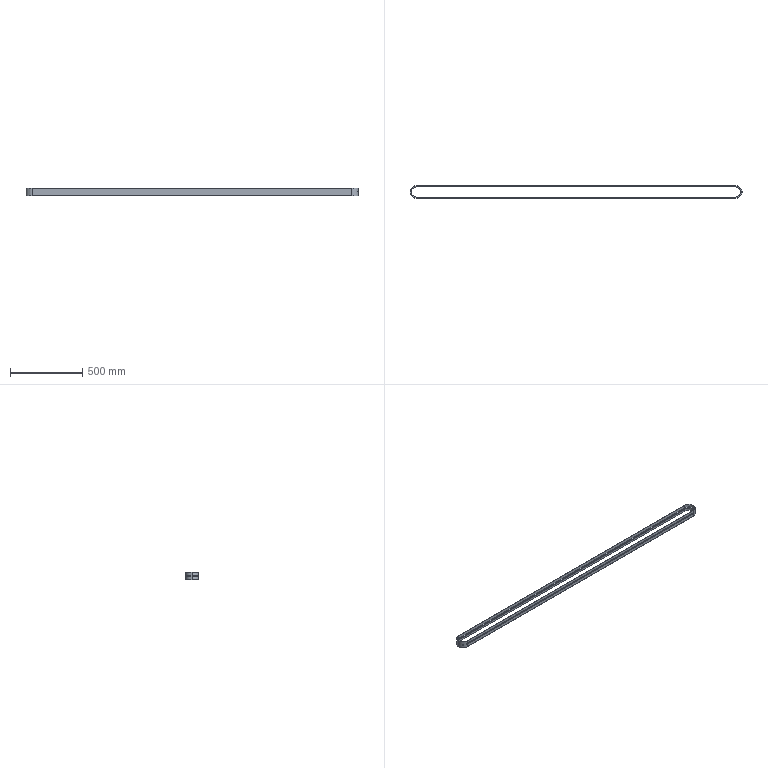Part | SolidWorks | features ExtruThin 1, Sweep 1 | 2 solids | 36 faces | box 2303 x 86 x 50 mm | volume 856015 mm3 | plane 18 | cylinder 12 | cone 6 | commonest cylinder face diameters 80 x6 70 x3 86 x3
STEP:
#1=CARTESIAN_POINT('',(-1108.5,40.,25.));
#2=VERTEX_POINT('',#1);
#3=CARTESIAN_POINT('',(-1148.5,0.,25.));
#4=VERTEX_POINT('',#3);
#5=CARTESIAN_POINT('',(-1108.5,0.,25.));
#6=DIRECTION('',(0.,0.,1.));
#7=DIRECTION('',(1.,0.,0.));
#8=AXIS2_PLACEMENT_3D('',#5,#6,#7);
#9=CIRCLE('',#8,40.);
#10=EDGE_CURVE('',#2,#4,#9,.T.);
#11=ORIENTED_EDGE('',*,*,#10,.T.);
#12=CARTESIAN_POINT('',(-1148.5,0.,-25.));
#13=VERTEX_POINT('',#12);
#14=CARTESIAN_POINT('',(-1148.5,0.,25.));
#15=DIRECTION('',(0.,0.,-1.));
#16=VECTOR('',#15,1000.);
#17=LINE('',#14,#16);
#18=EDGE_CURVE('',#4,#13,#17,.T.);
#19=ORIENTED_EDGE('',*,*,#18,.T.);
#20=CARTESIAN_POINT('',(-1108.5,40.,-25.));
#21=VERTEX_POINT('',#20);
#22=CARTESIAN_POINT('',(-1108.5,0.,-25.));
#23=DIRECTION('',(0.,0.,1.));
#24=DIRECTION('',(1.,0.,0.));
#25=AXIS2_PLACEMENT_3D('',#22,#23,#24);
#26=CIRCLE('',#25,40.);
#27=EDGE_CURVE('',#21,#13,#26,.T.);
#28=ORIENTED_EDGE('',*,*,#27,.F.);
#29=CARTESIAN_POINT('',(-1108.5,40.,25.));
#30=DIRECTION('',(0.,0.,-1.));
#31=VECTOR('',#30,1000.);
#32=LINE('',#29,#31);
#33=EDGE_CURVE('',#2,#21,#32,.T.);
#34=ORIENTED_EDGE('',*,*,#33,.F.);
#35=EDGE_LOOP('',(#11,#19,#28,#34));
#36=FACE_OUTER_BOUND('',#35,.T.);
#37=CARTESIAN_POINT('',(-1108.5,0.,25.));
#38=DIRECTION('',(0.,0.,-1.));
#39=DIRECTION('',(-1.,0.,0.));
#40=AXIS2_PLACEMENT_3D('',#37,#38,#39);
#41=CYLINDRICAL_SURFACE('',#40,40.);
#42=ADVANCED_FACE('',(#36),#41,.F.);
#43=CARTESIAN_POINT('',(-1151.5,0.,25.));
#44=VERTEX_POINT('',#43);
#45=CARTESIAN_POINT('',(-1108.5,-43.,25.));
#46=VERTEX_POINT('',#45);
#47=CARTESIAN_POINT('',(-1108.5,0.,25.));
#48=DIRECTION('',(0.,0.,1.));
#49=DIRECTION('',(1.,0.,0.));
#50=AXIS2_PLACEMENT_3D('',#47,#48,#49);
#51=CIRCLE('',#50,43.);
#52=EDGE_CURVE('',#44,#46,#51,.T.);
#53=ORIENTED_EDGE('',*,*,#52,.F.);
#54=CARTESIAN_POINT('',(-1151.5,0.,-25.));
#55=VERTEX_POINT('',#54);
#56=CARTESIAN_POINT('',(-1151.5,0.,25.));
#57=DIRECTION('',(0.,0.,-1.));
#58=VECTOR('',#57,1000.);
#59=LINE('',#56,#58);
#60=EDGE_CURVE('',#44,#55,#59,.T.);
#61=ORIENTED_EDGE('',*,*,#60,.T.);
#62=CARTESIAN_POINT('',(-1108.5,-43.,-25.));
#63=VERTEX_POINT('',#62);
#64=CARTESIAN_POINT('',(-1108.5,0.,-25.));
#65=DIRECTION('',(0.,0.,1.));
#66=DIRECTION('',(1.,0.,0.));
#67=AXIS2_PLACEMENT_3D('',#64,#65,#66);
#68=CIRCLE('',#67,43.);
#69=EDGE_CURVE('',#55,#63,#68,.T.);
#70=ORIENTED_EDGE('',*,*,#69,.T.);
#71=CARTESIAN_POINT('',(-1108.5,-43.,25.));
#72=DIRECTION('',(0.,0.,-1.));
#73=VECTOR('',#72,1000.);
#74=LINE('',#71,#73);
#75=EDGE_CURVE('',#46,#63,#74,.T.);
#76=ORIENTED_EDGE('',*,*,#75,.F.);
#77=EDGE_LOOP('',(#53,#61,#70,#76));
#78=FACE_OUTER_BOUND('',#77,.T.);
#79=CARTESIAN_POINT('',(-1108.5,0.,25.));
#80=DIRECTION('',(0.,0.,-1.));
#81=DIRECTION('',(-1.,0.,0.));
#82=AXIS2_PLACEMENT_3D('',#79,#80,#81);
#83=CYLINDRICAL_SURFACE('',#82,43.);
#84=ADVANCED_FACE('',(#78),#83,.T.);
#85=CARTESIAN_POINT('',(-1108.5,43.,25.));
#86=VERTEX_POINT('',#85);
#87=CARTESIAN_POINT('',(-1108.5,0.,25.));
#88=DIRECTION('',(0.,0.,1.));
#89=DIRECTION('',(1.,0.,0.));
#90=AXIS2_PLACEMENT_3D('',#87,#88,#89);
#91=CIRCLE('',#90,43.);
#92=EDGE_CURVE('',#86,#44,#91,.T.);
#93=ORIENTED_EDGE('',*,*,#92,.T.);
#94=ORIENTED_EDGE('',*,*,#52,.T.);
#95=CARTESIAN_POINT('',(1108.5,-43.,25.));
#96=VERTEX_POINT('',#95);
#97=CARTESIAN_POINT('',(-1108.5,-43.,25.));
#98=DIRECTION('',(1.,0.,0.));
#99=VECTOR('',#98,1000.);
#100=LINE('',#97,#99);
#101=EDGE_CURVE('',#46,#96,#100,.T.);
#102=ORIENTED_EDGE('',*,*,#101,.T.);
#103=CARTESIAN_POINT('',(1108.5,43.,25.));
#104=VERTEX_POINT('',#103);
#105=CARTESIAN_POINT('',(1108.5,0.,25.));
#106=DIRECTION('',(0.,0.,1.));
#107=DIRECTION('',(-1.,0.,0.));
#108=AXIS2_PLACEMENT_3D('',#105,#106,#107);
#109=CIRCLE('',#108,43.);
#110=EDGE_CURVE('',#96,#104,#109,.T.);
#111=ORIENTED_EDGE('',*,*,#110,.T.);
#112=CARTESIAN_POINT('',(-1108.5,43.,25.));
#113=DIRECTION('',(-1.,0.,0.));
#114=VECTOR('',#113,1000.);
#115=LINE('',#112,#114);
#116=EDGE_CURVE('',#104,#86,#115,.T.);
#117=ORIENTED_EDGE('',*,*,#116,.T.);
#118=EDGE_LOOP('',(#93,#94,#102,#111,#117));
#119=FACE_OUTER_BOUND('',#118,.T.);
#120=CARTESIAN_POINT('',(-1108.5,-40.,25.));
#121=VERTEX_POINT('',#120);
#122=CARTESIAN_POINT('',(1108.5,-40.,25.));
#123=VERTEX_POINT('',#122);
#124=CARTESIAN_POINT('',(-1108.5,-40.,25.));
#125=DIRECTION('',(1.,0.,0.));
#126=VECTOR('',#125,1000.);
#127=LINE('',#124,#126);
#128=EDGE_CURVE('',#121,#123,#127,.T.);
#129=ORIENTED_EDGE('',*,*,#128,.F.);
#130=CARTESIAN_POINT('',(-1108.5,0.,25.));
#131=DIRECTION('',(0.,0.,1.));
#132=DIRECTION('',(1.,0.,0.));
#133=AXIS2_PLACEMENT_3D('',#130,#131,#132);
#134=CIRCLE('',#133,40.);
#135=EDGE_CURVE('',#4,#121,#134,.T.);
#136=ORIENTED_EDGE('',*,*,#135,.F.);
#137=ORIENTED_EDGE('',*,*,#10,.F.);
#138=CARTESIAN_POINT('',(1108.5,40.,25.));
#139=VERTEX_POINT('',#138);
#140=CARTESIAN_POINT('',(-1108.5,40.,25.));
#141=DIRECTION('',(-1.,0.,0.));
#142=VECTOR('',#141,1000.);
#143=LINE('',#140,#142);
#144=EDGE_CURVE('',#139,#2,#143,.T.);
#145=ORIENTED_EDGE('',*,*,#144,.F.);
#146=CARTESIAN_POINT('',(1108.5,0.,25.));
#147=DIRECTION('',(0.,0.,1.));
#148=DIRECTION('',(1.,0.,0.));
#149=AXIS2_PLACEMENT_3D('',#146,#147,#148);
#150=CIRCLE('',#149,40.);
#151=EDGE_CURVE('',#123,#139,#150,.T.);
#152=ORIENTED_EDGE('',*,*,#151,.F.);
#153=EDGE_LOOP('',(#129,#136,#137,#145,#152));
#154=FACE_BOUND('',#153,.T.);
#155=CARTESIAN_POINT('',(-1108.5,0.,25.));
#156=DIRECTION('',(0.,0.,1.));
#157=DIRECTION('',(1.,0.,0.));
#158=AXIS2_PLACEMENT_3D('',#155,#156,#157);
#159=PLANE('',#158);
#160=ADVANCED_FACE('',(#119,#154),#159,.T.);
#161=CARTESIAN_POINT('',(-1108.5,43.,-25.));
#162=VERTEX_POINT('',#161);
#163=CARTESIAN_POINT('',(-1108.5,0.,-25.));
#164=DIRECTION('',(0.,0.,1.));
#165=DIRECTION('',(1.,0.,0.));
#166=AXIS2_PLACEMENT_3D('',#163,#164,#165);
#167=CIRCLE('',#166,43.);
#168=EDGE_CURVE('',#162,#55,#167,.T.);
#169=ORIENTED_EDGE('',*,*,#168,.F.);
#170=CARTESIAN_POINT('',(1108.5,43.,-25.));
#171=VERTEX_POINT('',#170);
#172=CARTESIAN_POINT('',(-1108.5,43.,-25.));
#173=DIRECTION('',(-1.,0.,0.));
#174=VECTOR('',#173,1000.);
#175=LINE('',#172,#174);
#176=EDGE_CURVE('',#171,#162,#175,.T.);
#177=ORIENTED_EDGE('',*,*,#176,.F.);
#178=CARTESIAN_POINT('',(1108.5,-43.,-25.));
#179=VERTEX_POINT('',#178);
#180=CARTESIAN_POINT('',(1108.5,0.,-25.));
#181=DIRECTION('',(0.,0.,1.));
#182=DIRECTION('',(-1.,0.,0.));
#183=AXIS2_PLACEMENT_3D('',#180,#181,#182);
#184=CIRCLE('',#183,43.);
#185=EDGE_CURVE('',#179,#171,#184,.T.);
#186=ORIENTED_EDGE('',*,*,#185,.F.);
#187=CARTESIAN_POINT('',(-1108.5,-43.,-25.));
#188=DIRECTION('',(1.,0.,0.));
#189=VECTOR('',#188,1000.);
#190=LINE('',#187,#189);
#191=EDGE_CURVE('',#63,#179,#190,.T.);
#192=ORIENTED_EDGE('',*,*,#191,.F.);
#193=ORIENTED_EDGE('',*,*,#69,.F.);
#194=EDGE_LOOP('',(#169,#177,#186,#192,#193));
#195=FACE_OUTER_BOUND('',#194,.T.);
#196=ORIENTED_EDGE('',*,*,#27,.T.);
#197=CARTESIAN_POINT('',(-1108.5,-40.,-25.));
#198=VERTEX_POINT('',#197);
#199=CARTESIAN_POINT('',(-1108.5,0.,-25.));
#200=DIRECTION('',(0.,0.,1.));
#201=DIRECTION('',(1.,0.,0.));
#202=AXIS2_PLACEMENT_3D('',#199,#200,#201);
#203=CIRCLE('',#202,40.);
#204=EDGE_CURVE('',#13,#198,#203,.T.);
#205=ORIENTED_EDGE('',*,*,#204,.T.);
#206=CARTESIAN_POINT('',(1108.5,-40.,-25.));
#207=VERTEX_POINT('',#206);
#208=CARTESIAN_POINT('',(-1108.5,-40.,-25.));
#209=DIRECTION('',(1.,0.,0.));
#210=VECTOR('',#209,1000.);
#211=LINE('',#208,#210);
#212=EDGE_CURVE('',#198,#207,#211,.T.);
#213=ORIENTED_EDGE('',*,*,#212,.T.);
#214=CARTESIAN_POINT('',(1108.5,40.,-25.));
#215=VERTEX_POINT('',#214);
#216=CARTESIAN_POINT('',(1108.5,0.,-25.));
#217=DIRECTION('',(0.,0.,1.));
#218=DIRECTION('',(1.,0.,0.));
#219=AXIS2_PLACEMENT_3D('',#216,#217,#218);
#220=CIRCLE('',#219,40.);
#221=EDGE_CURVE('',#207,#215,#220,.T.);
#222=ORIENTED_EDGE('',*,*,#221,.T.);
#223=CARTESIAN_POINT('',(-1108.5,40.,-25.));
#224=DIRECTION('',(-1.,0.,0.));
#225=VECTOR('',#224,1000.);
#226=LINE('',#223,#225);
#227=EDGE_CURVE('',#215,#21,#226,.T.);
#228=ORIENTED_EDGE('',*,*,#227,.T.);
#229=EDGE_LOOP('',(#196,#205,#213,#222,#228));
#230=FACE_BOUND('',#229,.T.);
#231=CARTESIAN_POINT('',(-1108.5,0.,-25.));
#232=DIRECTION('',(0.,0.,1.));
#233=DIRECTION('',(1.,0.,0.));
#234=AXIS2_PLACEMENT_3D('',#231,#232,#233);
#235=PLANE('',#234);
#236=ADVANCED_FACE('',(#195,#230),#235,.F.);
#237=ORIENTED_EDGE('',*,*,#60,.F.);
#238=ORIENTED_EDGE('',*,*,#92,.F.);
#239=CARTESIAN_POINT('',(-1108.5,43.,25.));
#240=DIRECTION('',(0.,0.,-1.));
#241=VECTOR('',#240,1000.);
#242=LINE('',#239,#241);
#243=EDGE_CURVE('',#86,#162,#242,.T.);
#244=ORIENTED_EDGE('',*,*,#243,.T.);
#245=ORIENTED_EDGE('',*,*,#168,.T.);
#246=EDGE_LOOP('',(#237,#238,#244,#245));
#247=FACE_OUTER_BOUND('',#246,.T.);
#248=CARTESIAN_POINT('',(-1108.5,0.,25.));
#249=DIRECTION('',(0.,0.,-1.));
#250=DIRECTION('',(-1.,0.,0.));
#251=AXIS2_PLACEMENT_3D('',#248,#249,#250);
#252=CYLINDRICAL_SURFACE('',#251,43.);
#253=ADVANCED_FACE('',(#247),#252,.T.);
#254=ORIENTED_EDGE('',*,*,#191,.T.);
#255=CARTESIAN_POINT('',(1108.5,-43.,25.));
#256=DIRECTION('',(0.,0.,-1.));
#257=VECTOR('',#256,1000.);
#258=LINE('',#255,#257);
#259=EDGE_CURVE('',#96,#179,#258,.T.);
#260=ORIENTED_EDGE('',*,*,#259,.F.);
#261=ORIENTED_EDGE('',*,*,#101,.F.);
#262=ORIENTED_EDGE('',*,*,#75,.T.);
#263=EDGE_LOOP('',(#254,#260,#261,#262));
#264=FACE_OUTER_BOUND('',#263,.T.);
#265=CARTESIAN_POINT('',(-1108.5,-43.,25.));
#266=DIRECTION('',(0.,1.,0.));
#267=DIRECTION('',(0.,0.,1.));
#268=AXIS2_PLACEMENT_3D('',#265,#266,#267);
#269=PLANE('',#268);
#270=ADVANCED_FACE('',(#264),#269,.F.);
#271=ORIENTED_EDGE('',*,*,#185,.T.);
#272=CARTESIAN_POINT('',(1108.5,43.,25.));
#273=DIRECTION('',(0.,0.,-1.));
#274=VECTOR('',#273,1000.);
#275=LINE('',#272,#274);
#276=EDGE_CURVE('',#104,#171,#275,.T.);
#277=ORIENTED_EDGE('',*,*,#276,.F.);
#278=ORIENTED_EDGE('',*,*,#110,.F.);
#279=ORIENTED_EDGE('',*,*,#259,.T.);
#280=EDGE_LOOP('',(#271,#277,#278,#279));
#281=FACE_OUTER_BOUND('',#280,.T.);
#282=CARTESIAN_POINT('',(1108.5,0.,25.));
#283=DIRECTION('',(0.,0.,-1.));
#284=DIRECTION('',(-1.,0.,0.));
#285=AXIS2_PLACEMENT_3D('',#282,#283,#284);
#286=CYLINDRICAL_SURFACE('',#285,43.);
#287=ADVANCED_FACE('',(#281),#286,.T.);
#288=ORIENTED_EDGE('',*,*,#176,.T.);
#289=ORIENTED_EDGE('',*,*,#243,.F.);
#290=ORIENTED_EDGE('',*,*,#116,.F.);
#291=ORIENTED_EDGE('',*,*,#276,.T.);
#292=EDGE_LOOP('',(#288,#289,#290,#291));
#293=FACE_OUTER_BOUND('',#292,.T.);
#294=CARTESIAN_POINT('',(-1108.5,43.,25.));
#295=DIRECTION('',(0.,-1.,0.));
#296=DIRECTION('',(0.,0.,-1.));
#297=AXIS2_PLACEMENT_3D('',#294,#295,#296);
#298=PLANE('',#297);
#299=ADVANCED_FACE('',(#293),#298,.F.);
#300=ORIENTED_EDGE('',*,*,#18,.F.);
#301=ORIENTED_EDGE('',*,*,#135,.T.);
#302=CARTESIAN_POINT('',(-1108.5,-40.,25.));
#303=DIRECTION('',(0.,0.,-1.));
#304=VECTOR('',#303,1000.);
#305=LINE('',#302,#304);
#306=EDGE_CURVE('',#121,#198,#305,.T.);
#307=ORIENTED_EDGE('',*,*,#306,.T.);
#308=ORIENTED_EDGE('',*,*,#204,.F.);
#309=EDGE_LOOP('',(#300,#301,#307,#308));
#310=FACE_OUTER_BOUND('',#309,.T.);
#311=CARTESIAN_POINT('',(-1108.5,0.,25.));
#312=DIRECTION('',(0.,0.,-1.));
#313=DIRECTION('',(-1.,0.,0.));
#314=AXIS2_PLACEMENT_3D('',#311,#312,#313);
#315=CYLINDRICAL_SURFACE('',#314,40.);
#316=ADVANCED_FACE('',(#310),#315,.F.);
#317=ORIENTED_EDGE('',*,*,#212,.F.);
#318=ORIENTED_EDGE('',*,*,#306,.F.);
#319=ORIENTED_EDGE('',*,*,#128,.T.);
#320=CARTESIAN_POINT('',(1108.5,-40.,25.));
#321=DIRECTION('',(0.,0.,-1.));
#322=VECTOR('',#321,1000.);
#323=LINE('',#320,#322);
#324=EDGE_CURVE('',#123,#207,#323,.T.);
#325=ORIENTED_EDGE('',*,*,#324,.T.);
#326=EDGE_LOOP('',(#317,#318,#319,#325));
#327=FACE_OUTER_BOUND('',#326,.T.);
#328=CARTESIAN_POINT('',(-1108.5,-40.,25.));
#329=DIRECTION('',(0.,1.,0.));
#330=DIRECTION('',(0.,0.,1.));
#331=AXIS2_PLACEMENT_3D('',#328,#329,#330);
#332=PLANE('',#331);
#333=ADVANCED_FACE('',(#327),#332,.T.);
#334=ORIENTED_EDGE('',*,*,#221,.F.);
#335=ORIENTED_EDGE('',*,*,#324,.F.);
#336=ORIENTED_EDGE('',*,*,#151,.T.);
#337=CARTESIAN_POINT('',(1108.5,40.,25.));
#338=DIRECTION('',(0.,0.,-1.));
#339=VECTOR('',#338,1000.);
#340=LINE('',#337,#339);
#341=EDGE_CURVE('',#139,#215,#340,.T.);
#342=ORIENTED_EDGE('',*,*,#341,.T.);
#343=EDGE_LOOP('',(#334,#335,#336,#342));
#344=FACE_OUTER_BOUND('',#343,.T.);
#345=CARTESIAN_POINT('',(1108.5,0.,25.));
#346=DIRECTION('',(0.,0.,-1.));
#347=DIRECTION('',(-1.,0.,0.));
#348=AXIS2_PLACEMENT_3D('',#345,#346,#347);
#349=CYLINDRICAL_SURFACE('',#348,40.);
#350=ADVANCED_FACE('',(#344),#349,.F.);
#351=ORIENTED_EDGE('',*,*,#227,.F.);
#352=ORIENTED_EDGE('',*,*,#341,.F.);
#353=ORIENTED_EDGE('',*,*,#144,.T.);
#354=ORIENTED_EDGE('',*,*,#33,.T.);
#355=EDGE_LOOP('',(#351,#352,#353,#354));
#356=FACE_OUTER_BOUND('',#355,.T.);
#357=CARTESIAN_POINT('',(-1108.5,40.,25.));
#358=DIRECTION('',(0.,-1.,0.));
#359=DIRECTION('',(0.,0.,-1.));
#360=AXIS2_PLACEMENT_3D('',#357,#358,#359);
#361=PLANE('',#360);
#362=ADVANCED_FACE('',(#356),#361,.T.);
#363=CLOSED_SHELL('',(#42,#84,#160,#236,#253,#270,#287,#299,#316,#333,#350,#362));
#364=MANIFOLD_SOLID_BREP('',#363);
#365=CARTESIAN_POINT('',(1108.5,35.,2.5));
#366=VERTEX_POINT('',#365);
#367=CARTESIAN_POINT('',(1143.5,0.,2.5));
#368=VERTEX_POINT('',#367);
#369=CARTESIAN_POINT('',(1108.5,0.,2.5));
#370=DIRECTION('',(0.,0.,-1.));
#371=DIRECTION('',(0.,1.,0.));
#372=AXIS2_PLACEMENT_3D('',#369,#370,#371);
#373=CIRCLE('',#372,35.);
#374=EDGE_CURVE('',#366,#368,#373,.T.);
#375=ORIENTED_EDGE('',*,*,#374,.T.);
#376=CARTESIAN_POINT('',(1148.5,0.,4.));
#377=VERTEX_POINT('',#376);
#378=CARTESIAN_POINT('',(1148.5,0.,4.));
#379=DIRECTION('',(0.9578,0.,0.2873));
#380=VECTOR('',#379,1000.);
#381=LINE('',#378,#380);
#382=EDGE_CURVE('',#368,#377,#381,.T.);
#383=ORIENTED_EDGE('',*,*,#382,.T.);
#384=CARTESIAN_POINT('',(1108.5,40.,4.));
#385=VERTEX_POINT('',#384);
#386=CARTESIAN_POINT('',(1108.5,0.,4.));
#387=DIRECTION('',(0.,0.,-1.));
#388=DIRECTION('',(0.,1.,0.));
#389=AXIS2_PLACEMENT_3D('',#386,#387,#388);
#390=CIRCLE('',#389,40.);
#391=EDGE_CURVE('',#385,#377,#390,.T.);
#392=ORIENTED_EDGE('',*,*,#391,.F.);
#393=CARTESIAN_POINT('',(1108.5,40.,4.));
#394=DIRECTION('',(0.,-0.9578,-0.2873));
#395=VECTOR('',#394,1000.);
#396=LINE('',#393,#395);
#397=EDGE_CURVE('',#385,#366,#396,.T.);
#398=ORIENTED_EDGE('',*,*,#397,.T.);
#399=EDGE_LOOP('',(#375,#383,#392,#398));
#400=FACE_OUTER_BOUND('',#399,.T.);
#401=CARTESIAN_POINT('',(1108.5,0.,4.));
#402=DIRECTION('',(0.,0.,1.));
#403=DIRECTION('',(1.,0.,0.));
#404=AXIS2_PLACEMENT_3D('',#401,#402,#403);
#405=CONICAL_SURFACE('',#404,40.,1.279);
#406=ADVANCED_FACE('',(#400),#405,.F.);
#407=CARTESIAN_POINT('',(-1143.5,0.,2.5));
#408=VERTEX_POINT('',#407);
#409=CARTESIAN_POINT('',(-1108.5,35.,2.5));
#410=VERTEX_POINT('',#409);
#411=CARTESIAN_POINT('',(-1108.5,0.,2.5));
#412=DIRECTION('',(0.,0.,-1.));
#413=DIRECTION('',(0.,-1.,0.));
#414=AXIS2_PLACEMENT_3D('',#411,#412,#413);
#415=CIRCLE('',#414,35.);
#416=EDGE_CURVE('',#408,#410,#415,.T.);
#417=ORIENTED_EDGE('',*,*,#416,.F.);
#418=CARTESIAN_POINT('',(-1143.5,0.,-2.5));
#419=VERTEX_POINT('',#418);
#420=CARTESIAN_POINT('',(-1143.5,0.,0.));
#421=DIRECTION('',(0.,0.,-1.));
#422=VECTOR('',#421,1000.);
#423=LINE('',#420,#422);
#424=EDGE_CURVE('',#408,#419,#423,.T.);
#425=ORIENTED_EDGE('',*,*,#424,.T.);
#426=CARTESIAN_POINT('',(-1108.5,35.,-2.5));
#427=VERTEX_POINT('',#426);
#428=CARTESIAN_POINT('',(-1108.5,0.,-2.5));
#429=DIRECTION('',(0.,0.,-1.));
#430=DIRECTION('',(0.,-1.,0.));
#431=AXIS2_PLACEMENT_3D('',#428,#429,#430);
#432=CIRCLE('',#431,35.);
#433=EDGE_CURVE('',#419,#427,#432,.T.);
#434=ORIENTED_EDGE('',*,*,#433,.T.);
#435=CARTESIAN_POINT('',(-1108.5,35.,2.5));
#436=DIRECTION('',(0.,0.,-1.));
#437=VECTOR('',#436,1000.);
#438=LINE('',#435,#437);
#439=EDGE_CURVE('',#410,#427,#438,.T.);
#440=ORIENTED_EDGE('',*,*,#439,.F.);
#441=EDGE_LOOP('',(#417,#425,#434,#440));
#442=FACE_OUTER_BOUND('',#441,.T.);
#443=CARTESIAN_POINT('',(-1108.5,0.,0.));
#444=DIRECTION('',(0.,0.,-1.));
#445=DIRECTION('',(-1.,0.,0.));
#446=AXIS2_PLACEMENT_3D('',#443,#444,#445);
#447=CYLINDRICAL_SURFACE('',#446,35.);
#448=ADVANCED_FACE('',(#442),#447,.F.);
#449=ORIENTED_EDGE('',*,*,#433,.F.);
#450=CARTESIAN_POINT('',(-1148.5,0.,-4.));
#451=VERTEX_POINT('',#450);
#452=CARTESIAN_POINT('',(-1143.5,0.,-2.5));
#453=DIRECTION('',(-0.9578,0.,-0.2873));
#454=VECTOR('',#453,1000.);
#455=LINE('',#452,#454);
#456=EDGE_CURVE('',#419,#451,#455,.T.);
#457=ORIENTED_EDGE('',*,*,#456,.T.);
#458=CARTESIAN_POINT('',(-1108.5,40.,-4.));
#459=VERTEX_POINT('',#458);
#460=CARTESIAN_POINT('',(-1108.5,0.,-4.));
#461=DIRECTION('',(0.,0.,-1.));
#462=DIRECTION('',(0.,-1.,0.));
#463=AXIS2_PLACEMENT_3D('',#460,#461,#462);
#464=CIRCLE('',#463,40.);
#465=EDGE_CURVE('',#451,#459,#464,.T.);
#466=ORIENTED_EDGE('',*,*,#465,.T.);
#467=CARTESIAN_POINT('',(-1108.5,40.,-4.));
#468=DIRECTION('',(0.,0.9578,-0.2873));
#469=VECTOR('',#468,1000.);
#470=LINE('',#467,#469);
#471=EDGE_CURVE('',#427,#459,#470,.T.);
#472=ORIENTED_EDGE('',*,*,#471,.F.);
#473=EDGE_LOOP('',(#449,#457,#466,#472));
#474=FACE_OUTER_BOUND('',#473,.T.);
#475=CARTESIAN_POINT('',(-1108.5,0.,-2.5));
#476=DIRECTION('',(0.,0.,-1.));
#477=DIRECTION('',(-1.,0.,0.));
#478=AXIS2_PLACEMENT_3D('',#475,#476,#477);
#479=CONICAL_SURFACE('',#478,35.,1.279);
#480=ADVANCED_FACE('',(#474),#479,.F.);
#481=CARTESIAN_POINT('',(-1108.5,-40.,4.));
#482=VERTEX_POINT('',#481);
#483=CARTESIAN_POINT('',(-1148.5,0.,4.));
#484=VERTEX_POINT('',#483);
#485=CARTESIAN_POINT('',(-1108.5,0.,4.));
#486=DIRECTION('',(0.,0.,-1.));
#487=DIRECTION('',(0.,-1.,0.));
#488=AXIS2_PLACEMENT_3D('',#485,#486,#487);
#489=CIRCLE('',#488,40.);
#490=EDGE_CURVE('',#482,#484,#489,.T.);
#491=ORIENTED_EDGE('',*,*,#490,.T.);
#492=CARTESIAN_POINT('',(-1148.5,0.,0.));
#493=DIRECTION('',(0.,0.,-1.));
#494=VECTOR('',#493,1000.);
#495=LINE('',#492,#494);
#496=EDGE_CURVE('',#484,#451,#495,.T.);
#497=ORIENTED_EDGE('',*,*,#496,.T.);
#498=CARTESIAN_POINT('',(-1108.5,-40.,-4.));
#499=VERTEX_POINT('',#498);
#500=CARTESIAN_POINT('',(-1108.5,0.,-4.));
#501=DIRECTION('',(0.,0.,-1.));
#502=DIRECTION('',(0.,-1.,0.));
#503=AXIS2_PLACEMENT_3D('',#500,#501,#502);
#504=CIRCLE('',#503,40.);
#505=EDGE_CURVE('',#499,#451,#504,.T.);
#506=ORIENTED_EDGE('',*,*,#505,.F.);
#507=CARTESIAN_POINT('',(-1108.5,-40.,-4.));
#508=DIRECTION('',(0.,0.,1.));
#509=VECTOR('',#508,1000.);
#510=LINE('',#507,#509);
#511=EDGE_CURVE('',#499,#482,#510,.T.);
#512=ORIENTED_EDGE('',*,*,#511,.T.);
#513=EDGE_LOOP('',(#491,#497,#506,#512));
#514=FACE_OUTER_BOUND('',#513,.T.);
#515=CARTESIAN_POINT('',(-1108.5,0.,0.));
#516=DIRECTION('',(0.,0.,-1.));
#517=DIRECTION('',(-1.,0.,0.));
#518=AXIS2_PLACEMENT_3D('',#515,#516,#517);
#519=CYLINDRICAL_SURFACE('',#518,40.);
#520=ADVANCED_FACE('',(#514),#519,.T.);
#521=CARTESIAN_POINT('',(-1108.5,40.,4.));
#522=VERTEX_POINT('',#521);
#523=CARTESIAN_POINT('',(0.,40.,4.));
#524=VERTEX_POINT('',#523);
#525=CARTESIAN_POINT('',(-1108.5,40.,4.));
#526=DIRECTION('',(1.,0.,0.));
#527=VECTOR('',#526,1000.);
#528=LINE('',#525,#527);
#529=EDGE_CURVE('',#522,#524,#528,.T.);
#530=ORIENTED_EDGE('',*,*,#529,.F.);
#531=CARTESIAN_POINT('',(-1108.5,40.,4.));
#532=DIRECTION('',(0.,-0.9578,-0.2873));
#533=VECTOR('',#532,1000.);
#534=LINE('',#531,#533);
#535=EDGE_CURVE('',#522,#410,#534,.T.);
#536=ORIENTED_EDGE('',*,*,#535,.T.);
#537=CARTESIAN_POINT('',(0.,35.,2.5));
#538=VERTEX_POINT('',#537);
#539=CARTESIAN_POINT('',(-1108.5,35.,2.5));
#540=DIRECTION('',(1.,0.,0.));
#541=VECTOR('',#540,1000.);
#542=LINE('',#539,#541);
#543=EDGE_CURVE('',#410,#538,#542,.T.);
#544=ORIENTED_EDGE('',*,*,#543,.T.);
#545=CARTESIAN_POINT('',(0.,40.,4.));
#546=DIRECTION('',(0.,-0.9578,-0.2873));
#547=VECTOR('',#546,1000.);
#548=LINE('',#545,#547);
#549=EDGE_CURVE('',#524,#538,#548,.T.);
#550=ORIENTED_EDGE('',*,*,#549,.F.);
#551=EDGE_LOOP('',(#530,#536,#544,#550));
#552=FACE_OUTER_BOUND('',#551,.T.);
#553=CARTESIAN_POINT('',(-1108.5,40.,4.));
#554=DIRECTION('',(0.,-0.2873,0.9578));
#555=DIRECTION('',(0.,-0.9578,-0.2873));
#556=AXIS2_PLACEMENT_3D('',#553,#554,#555);
#557=PLANE('',#556);
#558=ADVANCED_FACE('',(#552),#557,.T.);
#559=CARTESIAN_POINT('',(0.,40.,-4.));
#560=VERTEX_POINT('',#559);
#561=CARTESIAN_POINT('',(-1108.5,40.,-4.));
#562=DIRECTION('',(1.,0.,0.));
#563=VECTOR('',#562,1000.);
#564=LINE('',#561,#563);
#565=EDGE_CURVE('',#459,#560,#564,.T.);
#566=ORIENTED_EDGE('',*,*,#565,.F.);
#567=CARTESIAN_POINT('',(-1108.5,40.,-4.));
#568=DIRECTION('',(0.,0.,1.));
#569=VECTOR('',#568,1000.);
#570=LINE('',#567,#569);
#571=EDGE_CURVE('',#459,#522,#570,.T.);
#572=ORIENTED_EDGE('',*,*,#571,.T.);
#573=ORIENTED_EDGE('',*,*,#529,.T.);
#574=CARTESIAN_POINT('',(0.,40.,-4.));
#575=DIRECTION('',(0.,0.,1.));
#576=VECTOR('',#575,1000.);
#577=LINE('',#574,#576);
#578=EDGE_CURVE('',#560,#524,#577,.T.);
#579=ORIENTED_EDGE('',*,*,#578,.F.);
#580=EDGE_LOOP('',(#566,#572,#573,#579));
#581=FACE_OUTER_BOUND('',#580,.T.);
#582=CARTESIAN_POINT('',(-1108.5,40.,-4.));
#583=DIRECTION('',(0.,1.,0.));
#584=DIRECTION('',(0.,0.,1.));
#585=AXIS2_PLACEMENT_3D('',#582,#583,#584);
#586=PLANE('',#585);
#587=ADVANCED_FACE('',(#581),#586,.T.);
#588=CARTESIAN_POINT('',(0.,35.,-2.5));
#589=VERTEX_POINT('',#588);
#590=CARTESIAN_POINT('',(-1108.5,35.,-2.5));
#591=DIRECTION('',(1.,0.,0.));
#592=VECTOR('',#591,1000.);
#593=LINE('',#590,#592);
#594=EDGE_CURVE('',#427,#589,#593,.T.);
#595=ORIENTED_EDGE('',*,*,#594,.F.);
#596=ORIENTED_EDGE('',*,*,#471,.T.);
#597=ORIENTED_EDGE('',*,*,#565,.T.);
#598=CARTESIAN_POINT('',(0.,40.,-4.));
#599=DIRECTION('',(0.,0.9578,-0.2873));
#600=VECTOR('',#599,1000.);
#601=LINE('',#598,#600);
#602=EDGE_CURVE('',#589,#560,#601,.T.);
#603=ORIENTED_EDGE('',*,*,#602,.F.);
#604=EDGE_LOOP('',(#595,#596,#597,#603));
#605=FACE_OUTER_BOUND('',#604,.T.);
#606=CARTESIAN_POINT('',(-1108.5,40.,-4.));
#607=DIRECTION('',(0.,-0.2873,-0.9578));
#608=DIRECTION('',(0.,0.9578,-0.2873));
#609=AXIS2_PLACEMENT_3D('',#606,#607,#608);
#610=PLANE('',#609);
#611=ADVANCED_FACE('',(#605),#610,.T.);
#612=ORIENTED_EDGE('',*,*,#535,.F.);
#613=CARTESIAN_POINT('',(-1108.5,0.,4.));
#614=DIRECTION('',(0.,0.,-1.));
#615=DIRECTION('',(0.,-1.,0.));
#616=AXIS2_PLACEMENT_3D('',#613,#614,#615);
#617=CIRCLE('',#616,40.);
#618=EDGE_CURVE('',#484,#522,#617,.T.);
#619=ORIENTED_EDGE('',*,*,#618,.F.);
#620=ORIENTED_EDGE('',*,*,#490,.F.);
#621=CARTESIAN_POINT('',(-1108.5,-35.,2.5));
#622=VERTEX_POINT('',#621);
#623=CARTESIAN_POINT('',(-1108.5,-40.,4.));
#624=DIRECTION('',(0.,0.9578,-0.2873));
#625=VECTOR('',#624,1000.);
#626=LINE('',#623,#625);
#627=EDGE_CURVE('',#482,#622,#626,.T.);
#628=ORIENTED_EDGE('',*,*,#627,.T.);
#629=CARTESIAN_POINT('',(-1108.5,0.,2.5));
#630=DIRECTION('',(0.,0.,-1.));
#631=DIRECTION('',(0.,-1.,0.));
#632=AXIS2_PLACEMENT_3D('',#629,#630,#631);
#633=CIRCLE('',#632,35.);
#634=EDGE_CURVE('',#622,#408,#633,.T.);
#635=ORIENTED_EDGE('',*,*,#634,.T.);
#636=ORIENTED_EDGE('',*,*,#416,.T.);
#637=EDGE_LOOP('',(#612,#619,#620,#628,#635,#636));
#638=FACE_OUTER_BOUND('',#637,.T.);
#639=CARTESIAN_POINT('',(-1108.5,0.,4.));
#640=DIRECTION('',(0.,0.,1.));
#641=DIRECTION('',(1.,0.,0.));
#642=AXIS2_PLACEMENT_3D('',#639,#640,#641);
#643=CONICAL_SURFACE('',#642,40.,1.279);
#644=ADVANCED_FACE('',(#638),#643,.F.);
#645=ORIENTED_EDGE('',*,*,#496,.F.);
#646=ORIENTED_EDGE('',*,*,#618,.T.);
#647=ORIENTED_EDGE('',*,*,#571,.F.);
#648=ORIENTED_EDGE('',*,*,#465,.F.);
#649=EDGE_LOOP('',(#645,#646,#647,#648));
#650=FACE_OUTER_BOUND('',#649,.T.);
#651=CARTESIAN_POINT('',(-1108.5,0.,0.));
#652=DIRECTION('',(0.,0.,-1.));
#653=DIRECTION('',(-1.,0.,0.));
#654=AXIS2_PLACEMENT_3D('',#651,#652,#653);
#655=CYLINDRICAL_SURFACE('',#654,40.);
#656=ADVANCED_FACE('',(#650),#655,.T.);
#657=ORIENTED_EDGE('',*,*,#456,.F.);
#658=CARTESIAN_POINT('',(-1108.5,-35.,-2.5));
#659=VERTEX_POINT('',#658);
#660=CARTESIAN_POINT('',(-1108.5,0.,-2.5));
#661=DIRECTION('',(0.,0.,-1.));
#662=DIRECTION('',(0.,-1.,0.));
#663=AXIS2_PLACEMENT_3D('',#660,#661,#662);
#664=CIRCLE('',#663,35.);
#665=EDGE_CURVE('',#659,#419,#664,.T.);
#666=ORIENTED_EDGE('',*,*,#665,.F.);
#667=CARTESIAN_POINT('',(-1108.5,-40.,-4.));
#668=DIRECTION('',(0.,-0.9578,-0.2873));
#669=VECTOR('',#668,1000.);
#670=LINE('',#667,#669);
#671=EDGE_CURVE('',#659,#499,#670,.T.);
#672=ORIENTED_EDGE('',*,*,#671,.T.);
#673=ORIENTED_EDGE('',*,*,#505,.T.);
#674=EDGE_LOOP('',(#657,#666,#672,#673));
#675=FACE_OUTER_BOUND('',#674,.T.);
#676=CARTESIAN_POINT('',(-1108.5,0.,-2.5));
#677=DIRECTION('',(0.,0.,-1.));
#678=DIRECTION('',(-1.,0.,0.));
#679=AXIS2_PLACEMENT_3D('',#676,#677,#678);
#680=CONICAL_SURFACE('',#679,35.,1.279);
#681=ADVANCED_FACE('',(#675),#680,.F.);
#682=ORIENTED_EDGE('',*,*,#424,.F.);
#683=ORIENTED_EDGE('',*,*,#634,.F.);
#684=CARTESIAN_POINT('',(-1108.5,-35.,2.5));
#685=DIRECTION('',(0.,0.,-1.));
#686=VECTOR('',#685,1000.);
#687=LINE('',#684,#686);
#688=EDGE_CURVE('',#622,#659,#687,.T.);
#689=ORIENTED_EDGE('',*,*,#688,.T.);
#690=ORIENTED_EDGE('',*,*,#665,.T.);
#691=EDGE_LOOP('',(#682,#683,#689,#690));
#692=FACE_OUTER_BOUND('',#691,.T.);
#693=CARTESIAN_POINT('',(-1108.5,0.,0.));
#694=DIRECTION('',(0.,0.,-1.));
#695=DIRECTION('',(-1.,0.,0.));
#696=AXIS2_PLACEMENT_3D('',#693,#694,#695);
#697=CYLINDRICAL_SURFACE('',#696,35.);
#698=ADVANCED_FACE('',(#692),#697,.F.);
#699=ORIENTED_EDGE('',*,*,#627,.F.);
#700=CARTESIAN_POINT('',(1108.5,-40.,4.));
#701=VERTEX_POINT('',#700);
#702=CARTESIAN_POINT('',(1108.5,-40.,4.));
#703=DIRECTION('',(-1.,0.,0.));
#704=VECTOR('',#703,1000.);
#705=LINE('',#702,#704);
#706=EDGE_CURVE('',#701,#482,#705,.T.);
#707=ORIENTED_EDGE('',*,*,#706,.F.);
#708=CARTESIAN_POINT('',(1108.5,-35.,2.5));
#709=VERTEX_POINT('',#708);
#710=CARTESIAN_POINT('',(1108.5,-40.,4.));
#711=DIRECTION('',(0.,0.9578,-0.2873));
#712=VECTOR('',#711,1000.);
#713=LINE('',#710,#712);
#714=EDGE_CURVE('',#701,#709,#713,.T.);
#715=ORIENTED_EDGE('',*,*,#714,.T.);
#716=CARTESIAN_POINT('',(1108.5,-35.,2.5));
#717=DIRECTION('',(-1.,0.,0.));
#718=VECTOR('',#717,1000.);
#719=LINE('',#716,#718);
#720=EDGE_CURVE('',#709,#622,#719,.T.);
#721=ORIENTED_EDGE('',*,*,#720,.T.);
#722=EDGE_LOOP('',(#699,#707,#715,#721));
#723=FACE_OUTER_BOUND('',#722,.T.);
#724=CARTESIAN_POINT('',(1108.5,-40.,4.));
#725=DIRECTION('',(0.,0.2873,0.9578));
#726=DIRECTION('',(0.,-0.9578,0.2873));
#727=AXIS2_PLACEMENT_3D('',#724,#725,#726);
#728=PLANE('',#727);
#729=ADVANCED_FACE('',(#723),#728,.T.);
#730=ORIENTED_EDGE('',*,*,#706,.T.);
#731=ORIENTED_EDGE('',*,*,#511,.F.);
#732=CARTESIAN_POINT('',(1108.5,-40.,-4.));
#733=VERTEX_POINT('',#732);
#734=CARTESIAN_POINT('',(1108.5,-40.,-4.));
#735=DIRECTION('',(-1.,0.,0.));
#736=VECTOR('',#735,1000.);
#737=LINE('',#734,#736);
#738=EDGE_CURVE('',#733,#499,#737,.T.);
#739=ORIENTED_EDGE('',*,*,#738,.F.);
#740=CARTESIAN_POINT('',(1108.5,-40.,-4.));
#741=DIRECTION('',(0.,0.,1.));
#742=VECTOR('',#741,1000.);
#743=LINE('',#740,#742);
#744=EDGE_CURVE('',#733,#701,#743,.T.);
#745=ORIENTED_EDGE('',*,*,#744,.T.);
#746=EDGE_LOOP('',(#730,#731,#739,#745));
#747=FACE_OUTER_BOUND('',#746,.T.);
#748=CARTESIAN_POINT('',(1108.5,-40.,-4.));
#749=DIRECTION('',(0.,-1.,0.));
#750=DIRECTION('',(0.,0.,-1.));
#751=AXIS2_PLACEMENT_3D('',#748,#749,#750);
#752=PLANE('',#751);
#753=ADVANCED_FACE('',(#747),#752,.T.);
#754=ORIENTED_EDGE('',*,*,#738,.T.);
#755=ORIENTED_EDGE('',*,*,#671,.F.);
#756=CARTESIAN_POINT('',(1108.5,-35.,-2.5));
#757=VERTEX_POINT('',#756);
#758=CARTESIAN_POINT('',(1108.5,-35.,-2.5));
#759=DIRECTION('',(-1.,0.,0.));
#760=VECTOR('',#759,1000.);
#761=LINE('',#758,#760);
#762=EDGE_CURVE('',#757,#659,#761,.T.);
#763=ORIENTED_EDGE('',*,*,#762,.F.);
#764=CARTESIAN_POINT('',(1108.5,-40.,-4.));
#765=DIRECTION('',(0.,-0.9578,-0.2873));
#766=VECTOR('',#765,1000.);
#767=LINE('',#764,#766);
#768=EDGE_CURVE('',#757,#733,#767,.T.);
#769=ORIENTED_EDGE('',*,*,#768,.T.);
#770=EDGE_LOOP('',(#754,#755,#763,#769));
#771=FACE_OUTER_BOUND('',#770,.T.);
#772=CARTESIAN_POINT('',(1108.5,-40.,-4.));
#773=DIRECTION('',(0.,0.2873,-0.9578));
#774=DIRECTION('',(0.,0.9578,0.2873));
#775=AXIS2_PLACEMENT_3D('',#772,#773,#774);
#776=PLANE('',#775);
#777=ADVANCED_FACE('',(#771),#776,.T.);
#778=ORIENTED_EDGE('',*,*,#762,.T.);
#779=ORIENTED_EDGE('',*,*,#688,.F.);
#780=ORIENTED_EDGE('',*,*,#720,.F.);
#781=CARTESIAN_POINT('',(1108.5,-35.,2.5));
#782=DIRECTION('',(0.,0.,-1.));
#783=VECTOR('',#782,1000.);
#784=LINE('',#781,#783);
#785=EDGE_CURVE('',#709,#757,#784,.T.);
#786=ORIENTED_EDGE('',*,*,#785,.T.);
#787=EDGE_LOOP('',(#778,#779,#780,#786));
#788=FACE_OUTER_BOUND('',#787,.T.);
#789=CARTESIAN_POINT('',(1108.5,-35.,2.5));
#790=DIRECTION('',(0.,1.,0.));
#791=DIRECTION('',(0.,0.,1.));
#792=AXIS2_PLACEMENT_3D('',#789,#790,#791);
#793=PLANE('',#792);
#794=ADVANCED_FACE('',(#788),#793,.T.);
#795=ORIENTED_EDGE('',*,*,#382,.F.);
#796=CARTESIAN_POINT('',(1108.5,0.,2.5));
#797=DIRECTION('',(0.,0.,-1.));
#798=DIRECTION('',(0.,1.,0.));
#799=AXIS2_PLACEMENT_3D('',#796,#797,#798);
#800=CIRCLE('',#799,35.);
#801=EDGE_CURVE('',#368,#709,#800,.T.);
#802=ORIENTED_EDGE('',*,*,#801,.T.);
#803=ORIENTED_EDGE('',*,*,#714,.F.);
#804=CARTESIAN_POINT('',(1108.5,0.,4.));
#805=DIRECTION('',(0.,0.,-1.));
#806=DIRECTION('',(0.,1.,0.));
#807=AXIS2_PLACEMENT_3D('',#804,#805,#806);
#808=CIRCLE('',#807,40.);
#809=EDGE_CURVE('',#377,#701,#808,.T.);
#810=ORIENTED_EDGE('',*,*,#809,.F.);
#811=EDGE_LOOP('',(#795,#802,#803,#810));
#812=FACE_OUTER_BOUND('',#811,.T.);
#813=CARTESIAN_POINT('',(1108.5,0.,4.));
#814=DIRECTION('',(0.,0.,1.));
#815=DIRECTION('',(1.,0.,0.));
#816=AXIS2_PLACEMENT_3D('',#813,#814,#815);
#817=CONICAL_SURFACE('',#816,40.,1.279);
#818=ADVANCED_FACE('',(#812),#817,.F.);
#819=ORIENTED_EDGE('',*,*,#391,.T.);
#820=ORIENTED_EDGE('',*,*,#809,.T.);
#821=ORIENTED_EDGE('',*,*,#744,.F.);
#822=CARTESIAN_POINT('',(1108.5,40.,-4.));
#823=VERTEX_POINT('',#822);
#824=CARTESIAN_POINT('',(1108.5,0.,-4.));
#825=DIRECTION('',(0.,0.,-1.));
#826=DIRECTION('',(0.,1.,0.));
#827=AXIS2_PLACEMENT_3D('',#824,#825,#826);
#828=CIRCLE('',#827,40.);
#829=EDGE_CURVE('',#823,#733,#828,.T.);
#830=ORIENTED_EDGE('',*,*,#829,.F.);
#831=CARTESIAN_POINT('',(1108.5,40.,-4.));
#832=DIRECTION('',(0.,0.,1.));
#833=VECTOR('',#832,1000.);
#834=LINE('',#831,#833);
#835=EDGE_CURVE('',#823,#385,#834,.T.);
#836=ORIENTED_EDGE('',*,*,#835,.T.);
#837=EDGE_LOOP('',(#819,#820,#821,#830,#836));
#838=FACE_OUTER_BOUND('',#837,.T.);
#839=CARTESIAN_POINT('',(1108.5,0.,0.));
#840=DIRECTION('',(0.,0.,-1.));
#841=DIRECTION('',(-1.,0.,0.));
#842=AXIS2_PLACEMENT_3D('',#839,#840,#841);
#843=CYLINDRICAL_SURFACE('',#842,40.);
#844=ADVANCED_FACE('',(#838),#843,.T.);
#845=ORIENTED_EDGE('',*,*,#829,.T.);
#846=ORIENTED_EDGE('',*,*,#768,.F.);
#847=CARTESIAN_POINT('',(1108.5,35.,-2.5));
#848=VERTEX_POINT('',#847);
#849=CARTESIAN_POINT('',(1108.5,0.,-2.5));
#850=DIRECTION('',(0.,0.,-1.));
#851=DIRECTION('',(0.,1.,0.));
#852=AXIS2_PLACEMENT_3D('',#849,#850,#851);
#853=CIRCLE('',#852,35.);
#854=EDGE_CURVE('',#848,#757,#853,.T.);
#855=ORIENTED_EDGE('',*,*,#854,.F.);
#856=CARTESIAN_POINT('',(1108.5,40.,-4.));
#857=DIRECTION('',(0.,0.9578,-0.2873));
#858=VECTOR('',#857,1000.);
#859=LINE('',#856,#858);
#860=EDGE_CURVE('',#848,#823,#859,.T.);
#861=ORIENTED_EDGE('',*,*,#860,.T.);
#862=EDGE_LOOP('',(#845,#846,#855,#861));
#863=FACE_OUTER_BOUND('',#862,.T.);
#864=CARTESIAN_POINT('',(1108.5,0.,-2.5));
#865=DIRECTION('',(0.,0.,-1.));
#866=DIRECTION('',(-1.,0.,0.));
#867=AXIS2_PLACEMENT_3D('',#864,#865,#866);
#868=CONICAL_SURFACE('',#867,35.,1.279);
#869=ADVANCED_FACE('',(#863),#868,.F.);
#870=ORIENTED_EDGE('',*,*,#854,.T.);
#871=ORIENTED_EDGE('',*,*,#785,.F.);
#872=ORIENTED_EDGE('',*,*,#801,.F.);
#873=ORIENTED_EDGE('',*,*,#374,.F.);
#874=CARTESIAN_POINT('',(1108.5,35.,2.5));
#875=DIRECTION('',(0.,0.,-1.));
#876=VECTOR('',#875,1000.);
#877=LINE('',#874,#876);
#878=EDGE_CURVE('',#366,#848,#877,.T.);
#879=ORIENTED_EDGE('',*,*,#878,.T.);
#880=EDGE_LOOP('',(#870,#871,#872,#873,#879));
#881=FACE_OUTER_BOUND('',#880,.T.);
#882=CARTESIAN_POINT('',(1108.5,0.,0.));
#883=DIRECTION('',(0.,0.,-1.));
#884=DIRECTION('',(-1.,0.,0.));
#885=AXIS2_PLACEMENT_3D('',#882,#883,#884);
#886=CYLINDRICAL_SURFACE('',#885,35.);
#887=ADVANCED_FACE('',(#881),#886,.F.);
#888=ORIENTED_EDGE('',*,*,#397,.F.);
#889=CARTESIAN_POINT('',(0.,40.,4.));
#890=DIRECTION('',(1.,0.,0.));
#891=VECTOR('',#890,1000.);
#892=LINE('',#889,#891);
#893=EDGE_CURVE('',#524,#385,#892,.T.);
#894=ORIENTED_EDGE('',*,*,#893,.F.);
#895=ORIENTED_EDGE('',*,*,#549,.T.);
#896=CARTESIAN_POINT('',(0.,35.,2.5));
#897=DIRECTION('',(1.,0.,0.));
#898=VECTOR('',#897,1000.);
#899=LINE('',#896,#898);
#900=EDGE_CURVE('',#538,#366,#899,.T.);
#901=ORIENTED_EDGE('',*,*,#900,.T.);
#902=EDGE_LOOP('',(#888,#894,#895,#901));
#903=FACE_OUTER_BOUND('',#902,.T.);
#904=CARTESIAN_POINT('',(0.,40.,4.));
#905=DIRECTION('',(0.,-0.2873,0.9578));
#906=DIRECTION('',(0.,-0.9578,-0.2873));
#907=AXIS2_PLACEMENT_3D('',#904,#905,#906);
#908=PLANE('',#907);
#909=ADVANCED_FACE('',(#903),#908,.T.);
#910=ORIENTED_EDGE('',*,*,#893,.T.);
#911=ORIENTED_EDGE('',*,*,#835,.F.);
#912=CARTESIAN_POINT('',(0.,40.,-4.));
#913=DIRECTION('',(1.,0.,0.));
#914=VECTOR('',#913,1000.);
#915=LINE('',#912,#914);
#916=EDGE_CURVE('',#560,#823,#915,.T.);
#917=ORIENTED_EDGE('',*,*,#916,.F.);
#918=ORIENTED_EDGE('',*,*,#578,.T.);
#919=EDGE_LOOP('',(#910,#911,#917,#918));
#920=FACE_OUTER_BOUND('',#919,.T.);
#921=CARTESIAN_POINT('',(0.,40.,-4.));
#922=DIRECTION('',(0.,1.,0.));
#923=DIRECTION('',(0.,0.,1.));
#924=AXIS2_PLACEMENT_3D('',#921,#922,#923);
#925=PLANE('',#924);
#926=ADVANCED_FACE('',(#920),#925,.T.);
#927=ORIENTED_EDGE('',*,*,#916,.T.);
#928=ORIENTED_EDGE('',*,*,#860,.F.);
#929=CARTESIAN_POINT('',(0.,35.,-2.5));
#930=DIRECTION('',(1.,0.,0.));
#931=VECTOR('',#930,1000.);
#932=LINE('',#929,#931);
#933=EDGE_CURVE('',#589,#848,#932,.T.);
#934=ORIENTED_EDGE('',*,*,#933,.F.);
#935=ORIENTED_EDGE('',*,*,#602,.T.);
#936=EDGE_LOOP('',(#927,#928,#934,#935));
#937=FACE_OUTER_BOUND('',#936,.T.);
#938=CARTESIAN_POINT('',(0.,40.,-4.));
#939=DIRECTION('',(0.,-0.2873,-0.9578));
#940=DIRECTION('',(0.,0.9578,-0.2873));
#941=AXIS2_PLACEMENT_3D('',#938,#939,#940);
#942=PLANE('',#941);
#943=ADVANCED_FACE('',(#937),#942,.T.);
#944=ORIENTED_EDGE('',*,*,#933,.T.);
#945=ORIENTED_EDGE('',*,*,#878,.F.);
#946=ORIENTED_EDGE('',*,*,#900,.F.);
#947=CARTESIAN_POINT('',(0.,35.,2.5));
#948=DIRECTION('',(0.,0.,-1.));
#949=VECTOR('',#948,1000.);
#950=LINE('',#947,#949);
#951=EDGE_CURVE('',#538,#589,#950,.T.);
#952=ORIENTED_EDGE('',*,*,#951,.T.);
#953=EDGE_LOOP('',(#944,#945,#946,#952));
#954=FACE_OUTER_BOUND('',#953,.T.);
#955=CARTESIAN_POINT('',(0.,35.,2.5));
#956=DIRECTION('',(0.,-1.,0.));
#957=DIRECTION('',(0.,0.,-1.));
#958=AXIS2_PLACEMENT_3D('',#955,#956,#957);
#959=PLANE('',#958);
#960=ADVANCED_FACE('',(#954),#959,.T.);
#961=ORIENTED_EDGE('',*,*,#439,.T.);
#962=ORIENTED_EDGE('',*,*,#594,.T.);
#963=ORIENTED_EDGE('',*,*,#951,.F.);
#964=ORIENTED_EDGE('',*,*,#543,.F.);
#965=EDGE_LOOP('',(#961,#962,#963,#964));
#966=FACE_OUTER_BOUND('',#965,.T.);
#967=CARTESIAN_POINT('',(-1108.5,35.,2.5));
#968=DIRECTION('',(0.,-1.,0.));
#969=DIRECTION('',(0.,0.,-1.));
#970=AXIS2_PLACEMENT_3D('',#967,#968,#969);
#971=PLANE('',#970);
#972=ADVANCED_FACE('',(#966),#971,.T.);
#973=CLOSED_SHELL('',(#406,#448,#480,#520,#558,#587,#611,#644,#656,#681,#698,#729,#753,#777,#794,#818,#844,#869,#887,#909,#926,#943,#960,#972));
#974=MANIFOLD_SOLID_BREP('',#973);
#975=CARTESIAN_POINT('',(0.,0.,0.));
#976=DIRECTION('',(0.,0.,1.));
#977=DIRECTION('',(1.,0.,0.));
#978=AXIS2_PLACEMENT_3D('',#975,#976,#977);
#979=(LENGTH_UNIT()NAMED_UNIT(*)SI_UNIT(.MILLI.,.METRE.));
#980=UNCERTAINTY_MEASURE_WITH_UNIT(LENGTH_MEASURE(0.00001),#979,'','');
#981=(NAMED_UNIT(*)PLANE_ANGLE_UNIT()SI_UNIT($,.RADIAN.));
#982=(NAMED_UNIT(*)SI_UNIT($,.STERADIAN.)SOLID_ANGLE_UNIT());
#983=(GEOMETRIC_REPRESENTATION_CONTEXT(3)GLOBAL_UNCERTAINTY_ASSIGNED_CONTEXT((#980))GLOBAL_UNIT_ASSIGNED_CONTEXT((#979,#981,#982))REPRESENTATION_CONTEXT('',''));
#984=ADVANCED_BREP_SHAPE_REPRESENTATION('',(#364,#974,#978),#983);